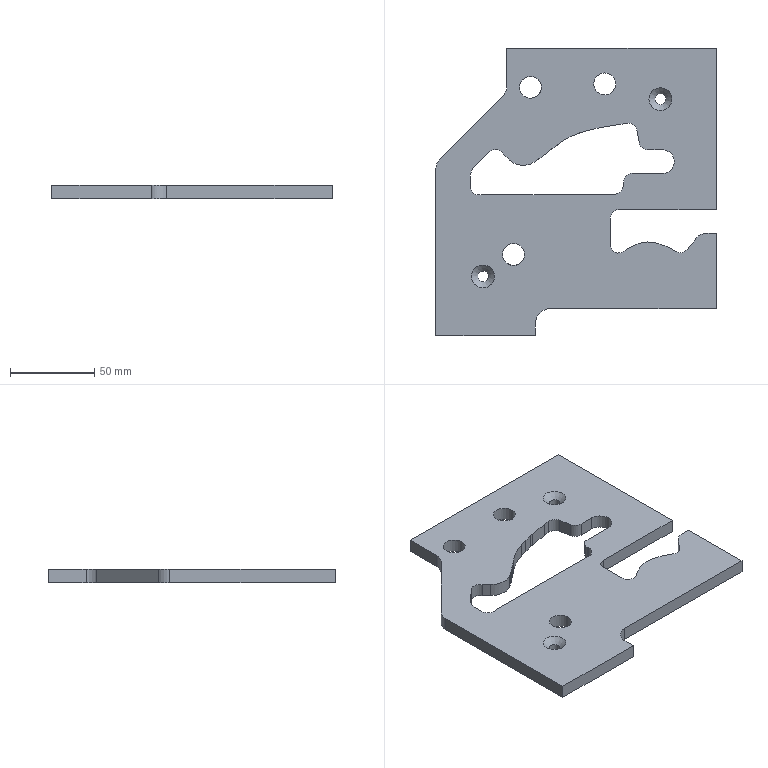Part | STEP file | gslz 2016.10.28-13_id138_x_t | 1 solid | 63 faces | box 166 x 170 x 8 mm | volume 157152 mm3 | plane 37 | cylinder 24 | cone 2 | commonest cylinder face diameters 10 x8 13 x3 18 x3 6.5 x2 14 x2 12 x1